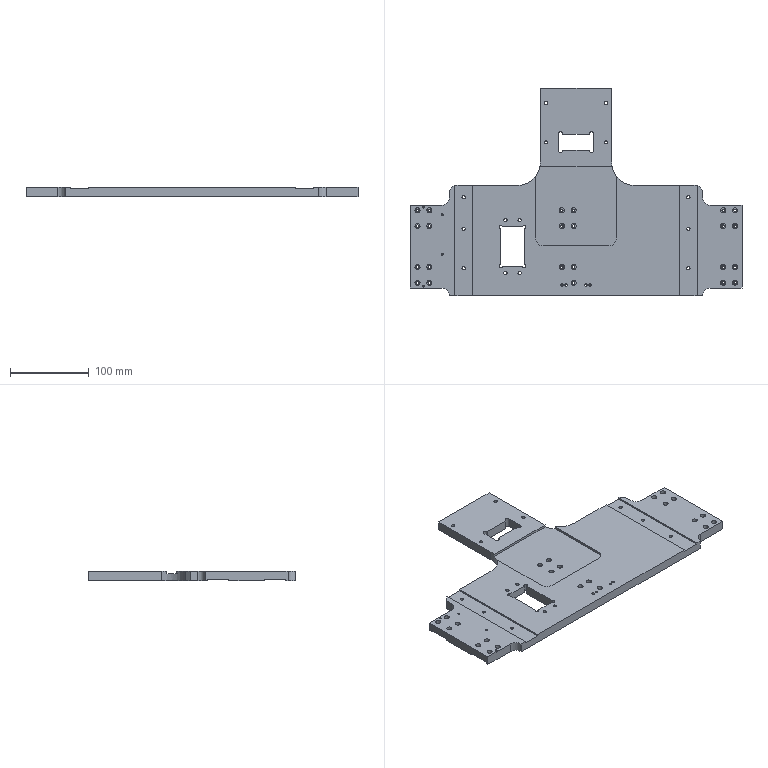Part | 1 solid | 250 faces | box 421 x 263.5 x 12 mm | volume 677810 mm3 | cylinder 158 | plane 78 | cone 14 | commonest cylinder face diameters 3.4 x46 6.5 x46 4.2 x32 2.5 x8 4 x6 20 x6